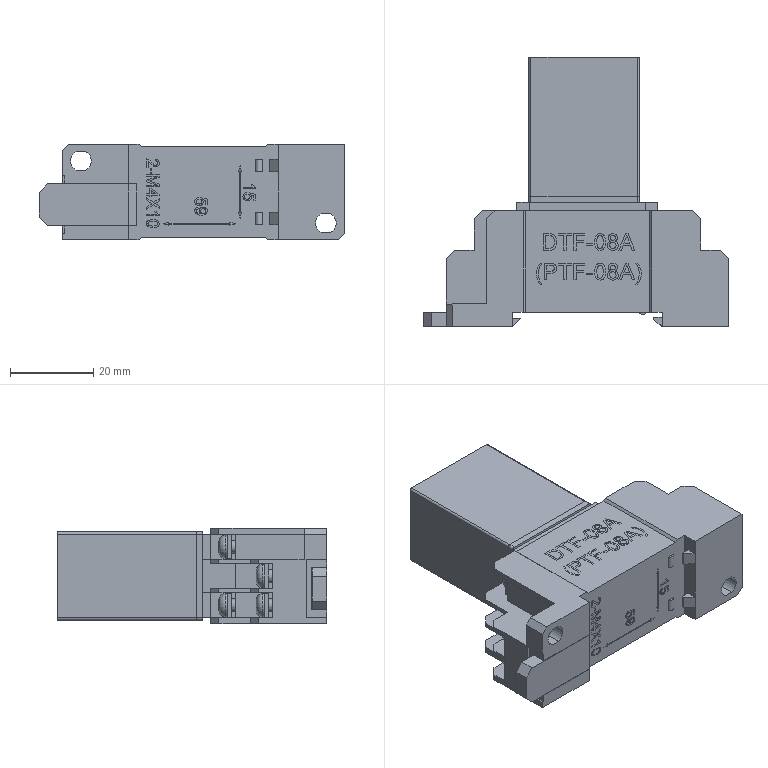Part | STEP file | LY2N - J _ DTF-08A ( PTF-08A )-1.step | 19 solids | 1494 faces | box 73.5 x 65 x 23.1 mm | volume 52348 mm3 | plane 982 | spline 410 | cylinder 86 | torus 16 | commonest cylinder face diameters 3 x16 3.5 x16 5.6 x16 1 x12 5 x6 0.94 x4